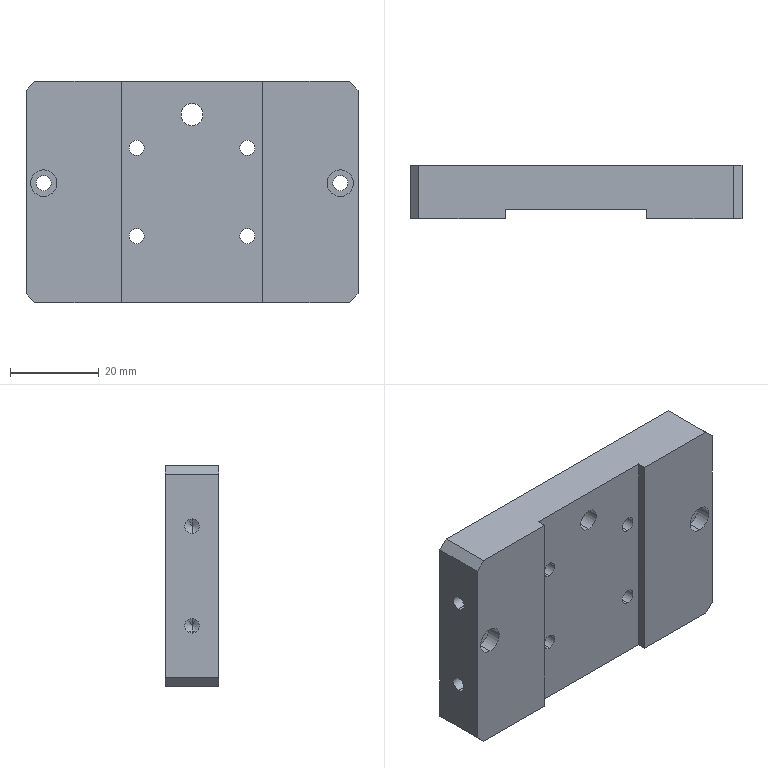Part | STEP file | PN_0005 | 1 solid | 62 faces | box 75 x 12 x 50 mm | volume 40001 mm3 | cylinder 34 | plane 20 | cone 8 | commonest cylinder face diameters 3.4 x12 6 x12 3.3 x4 4.2 x4 5 x2